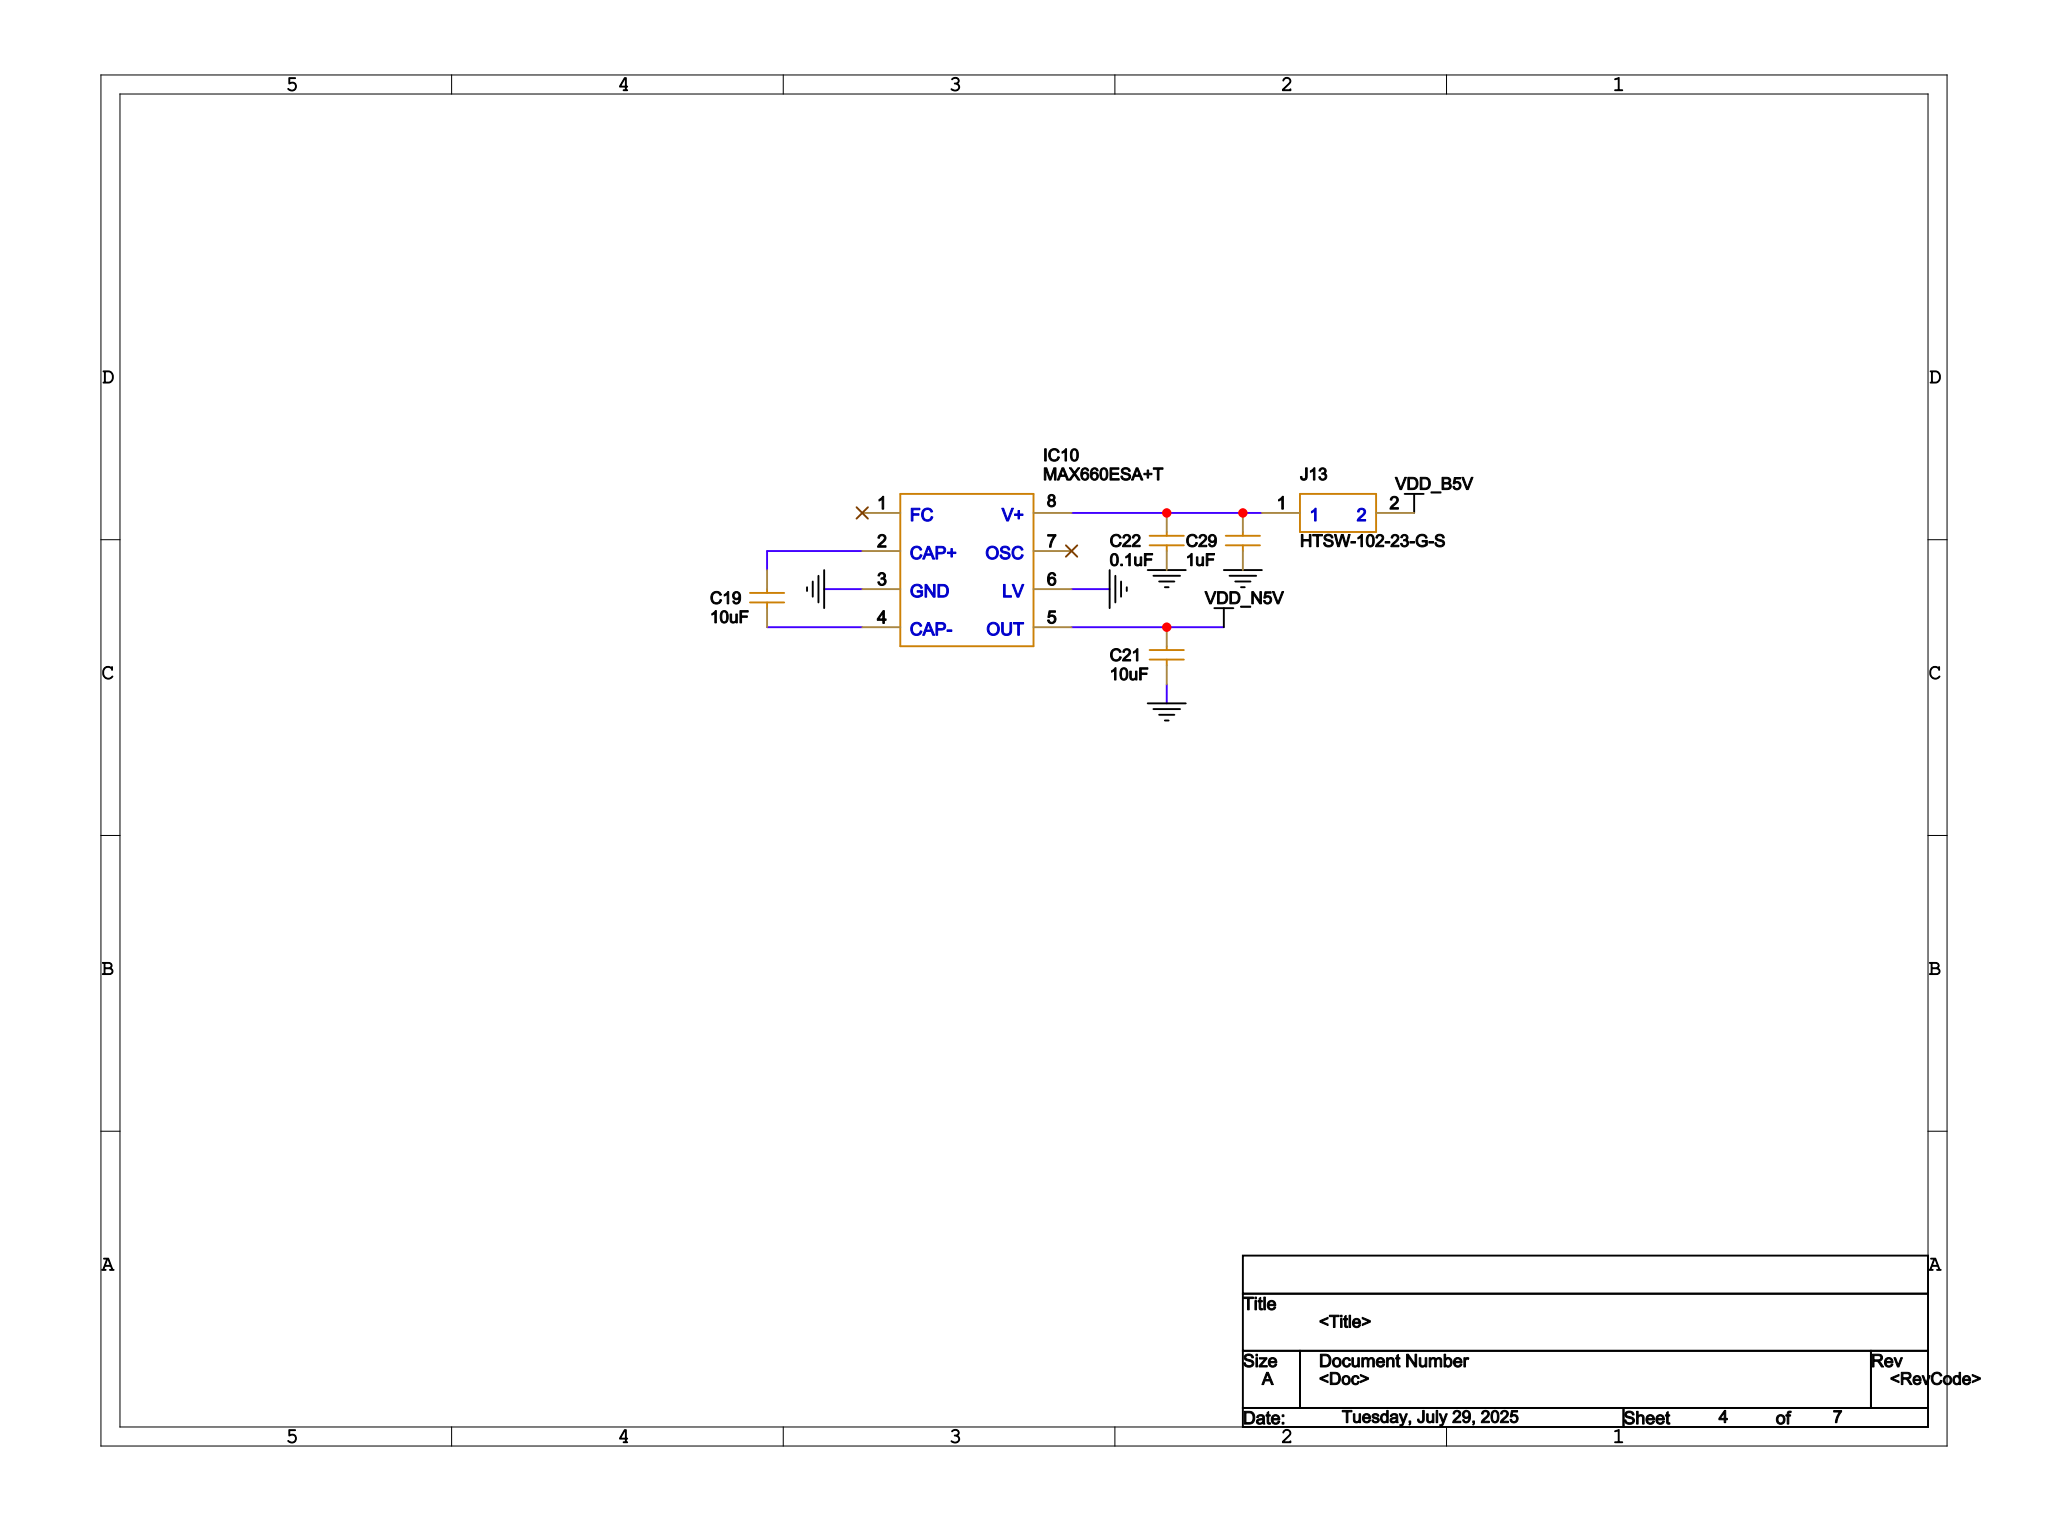Circuit board | Cadence Allegro | 93 parts | 49 nets | one sheet of the schematic
Parts on this sheet (reference | value | footprint):
C19 | 10uF | C1210
C21 | 10uF | C1210
C22 | 0.1uF | C0402
C29 | 1uF | C0402
IC10 | MAX660ESA+T | SOIC127P600X175-8N
J13 | HTSW-102-23-G-S | HDRV2W64P0X254_1X2_508X248X838P
Nets of these parts (net: part-pin ...):
GND: C21-2 C22-2 C29-2 IC10-3 IC10-6
VDD_B5V: J13-2
N08677: C19-1 IC10-2
N08684: C19-2 IC10-4
VDD_N5V: C21-1 IC10-5
N07934: C22-1 C29-1 IC10-8 J13-1